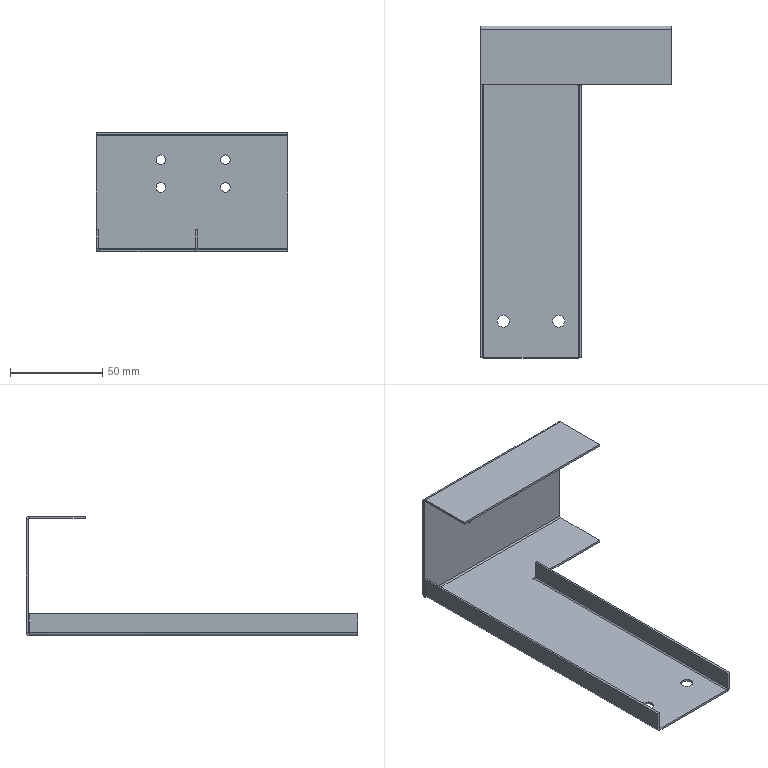Part | 1 solid | 54 faces | box 103.8 x 180 x 65 mm | volume 29196 mm3 | plane 34 | cylinder 20 | commonest cylinder face diameters 5.2 x8 1.473 x4 3.873 x4 6.5 x4
STEP:
#1=CARTESIAN_POINT('',(42.5,88.8,46.2));
#2=VERTEX_POINT('',#1);
#3=CARTESIAN_POINT('',(42.5,88.8,51.4));
#4=VERTEX_POINT('',#3);
#5=CARTESIAN_POINT('',(42.5,88.8,48.8));
#6=DIRECTION('',(0.,1.,0.));
#7=DIRECTION('',(0.,0.,1.));
#8=AXIS2_PLACEMENT_3D('',#5,#6,#7);
#9=CIRCLE('',#8,2.6);
#10=EDGE_CURVE('',#2,#4,#9,.T.);
#11=ORIENTED_EDGE('',*,*,#10,.F.);
#12=CARTESIAN_POINT('',(42.5,90.,46.2));
#13=VERTEX_POINT('',#12);
#14=CARTESIAN_POINT('',(42.5,80.,46.2));
#15=DIRECTION('',(0.,1.,0.));
#16=VECTOR('',#15,1000.);
#17=LINE('',#14,#16);
#18=EDGE_CURVE('',#2,#13,#17,.T.);
#19=ORIENTED_EDGE('',*,*,#18,.T.);
#20=CARTESIAN_POINT('',(42.5,90.,51.4));
#21=VERTEX_POINT('',#20);
#22=CARTESIAN_POINT('',(42.5,90.,48.8));
#23=DIRECTION('',(0.,1.,0.));
#24=DIRECTION('',(0.,0.,1.));
#25=AXIS2_PLACEMENT_3D('',#22,#23,#24);
#26=CIRCLE('',#25,2.6);
#27=EDGE_CURVE('',#13,#21,#26,.T.);
#28=ORIENTED_EDGE('',*,*,#27,.T.);
#29=CARTESIAN_POINT('',(42.5,80.,51.4));
#30=DIRECTION('',(0.,1.,0.));
#31=VECTOR('',#30,1000.);
#32=LINE('',#29,#31);
#33=EDGE_CURVE('',#4,#21,#32,.T.);
#34=ORIENTED_EDGE('',*,*,#33,.F.);
#35=EDGE_LOOP('',(#11,#19,#28,#34));
#36=FACE_OUTER_BOUND('',#35,.T.);
#37=CARTESIAN_POINT('',(42.5,80.,48.8));
#38=DIRECTION('',(0.,1.,0.));
#39=DIRECTION('',(0.,0.,1.));
#40=AXIS2_PLACEMENT_3D('',#37,#38,#39);
#41=CYLINDRICAL_SURFACE('',#40,2.6);
#42=ADVANCED_FACE('',(#36),#41,.F.);
#43=CARTESIAN_POINT('',(7.5,88.8,46.2));
#44=VERTEX_POINT('',#43);
#45=CARTESIAN_POINT('',(7.5,88.8,51.4));
#46=VERTEX_POINT('',#45);
#47=CARTESIAN_POINT('',(7.5,88.8,48.8));
#48=DIRECTION('',(0.,1.,0.));
#49=DIRECTION('',(0.,0.,1.));
#50=AXIS2_PLACEMENT_3D('',#47,#48,#49);
#51=CIRCLE('',#50,2.6);
#52=EDGE_CURVE('',#44,#46,#51,.T.);
#53=ORIENTED_EDGE('',*,*,#52,.F.);
#54=CARTESIAN_POINT('',(7.5,90.,46.2));
#55=VERTEX_POINT('',#54);
#56=CARTESIAN_POINT('',(7.5,80.,46.2));
#57=DIRECTION('',(0.,1.,0.));
#58=VECTOR('',#57,1000.);
#59=LINE('',#56,#58);
#60=EDGE_CURVE('',#44,#55,#59,.T.);
#61=ORIENTED_EDGE('',*,*,#60,.T.);
#62=CARTESIAN_POINT('',(7.5,90.,51.4));
#63=VERTEX_POINT('',#62);
#64=CARTESIAN_POINT('',(7.5,90.,48.8));
#65=DIRECTION('',(0.,1.,0.));
#66=DIRECTION('',(0.,0.,1.));
#67=AXIS2_PLACEMENT_3D('',#64,#65,#66);
#68=CIRCLE('',#67,2.6);
#69=EDGE_CURVE('',#55,#63,#68,.T.);
#70=ORIENTED_EDGE('',*,*,#69,.T.);
#71=CARTESIAN_POINT('',(7.5,80.,51.4));
#72=DIRECTION('',(0.,1.,0.));
#73=VECTOR('',#72,1000.);
#74=LINE('',#71,#73);
#75=EDGE_CURVE('',#46,#63,#74,.T.);
#76=ORIENTED_EDGE('',*,*,#75,.F.);
#77=EDGE_LOOP('',(#53,#61,#70,#76));
#78=FACE_OUTER_BOUND('',#77,.T.);
#79=CARTESIAN_POINT('',(7.5,80.,48.8));
#80=DIRECTION('',(0.,1.,0.));
#81=DIRECTION('',(0.,0.,1.));
#82=AXIS2_PLACEMENT_3D('',#79,#80,#81);
#83=CYLINDRICAL_SURFACE('',#82,2.6);
#84=ADVANCED_FACE('',(#78),#83,.F.);
#85=CARTESIAN_POINT('',(7.5,88.8,31.2));
#86=VERTEX_POINT('',#85);
#87=CARTESIAN_POINT('',(7.5,88.8,36.4));
#88=VERTEX_POINT('',#87);
#89=CARTESIAN_POINT('',(7.5,88.8,33.8));
#90=DIRECTION('',(0.,1.,0.));
#91=DIRECTION('',(0.,0.,1.));
#92=AXIS2_PLACEMENT_3D('',#89,#90,#91);
#93=CIRCLE('',#92,2.6);
#94=EDGE_CURVE('',#86,#88,#93,.T.);
#95=ORIENTED_EDGE('',*,*,#94,.F.);
#96=CARTESIAN_POINT('',(7.5,90.,31.2));
#97=VERTEX_POINT('',#96);
#98=CARTESIAN_POINT('',(7.5,80.,31.2));
#99=DIRECTION('',(0.,1.,0.));
#100=VECTOR('',#99,1000.);
#101=LINE('',#98,#100);
#102=EDGE_CURVE('',#86,#97,#101,.T.);
#103=ORIENTED_EDGE('',*,*,#102,.T.);
#104=CARTESIAN_POINT('',(7.5,90.,36.4));
#105=VERTEX_POINT('',#104);
#106=CARTESIAN_POINT('',(7.5,90.,33.8));
#107=DIRECTION('',(0.,1.,0.));
#108=DIRECTION('',(0.,0.,1.));
#109=AXIS2_PLACEMENT_3D('',#106,#107,#108);
#110=CIRCLE('',#109,2.6);
#111=EDGE_CURVE('',#97,#105,#110,.T.);
#112=ORIENTED_EDGE('',*,*,#111,.T.);
#113=CARTESIAN_POINT('',(7.5,80.,36.4));
#114=DIRECTION('',(0.,1.,0.));
#115=VECTOR('',#114,1000.);
#116=LINE('',#113,#115);
#117=EDGE_CURVE('',#88,#105,#116,.T.);
#118=ORIENTED_EDGE('',*,*,#117,.F.);
#119=EDGE_LOOP('',(#95,#103,#112,#118));
#120=FACE_OUTER_BOUND('',#119,.T.);
#121=CARTESIAN_POINT('',(7.5,80.,33.8));
#122=DIRECTION('',(0.,1.,0.));
#123=DIRECTION('',(0.,0.,1.));
#124=AXIS2_PLACEMENT_3D('',#121,#122,#123);
#125=CYLINDRICAL_SURFACE('',#124,2.6);
#126=ADVANCED_FACE('',(#120),#125,.F.);
#127=CARTESIAN_POINT('',(42.5,88.8,31.2));
#128=VERTEX_POINT('',#127);
#129=CARTESIAN_POINT('',(42.5,88.8,36.4));
#130=VERTEX_POINT('',#129);
#131=CARTESIAN_POINT('',(42.5,88.8,33.8));
#132=DIRECTION('',(0.,1.,0.));
#133=DIRECTION('',(0.,0.,1.));
#134=AXIS2_PLACEMENT_3D('',#131,#132,#133);
#135=CIRCLE('',#134,2.6);
#136=EDGE_CURVE('',#128,#130,#135,.T.);
#137=ORIENTED_EDGE('',*,*,#136,.F.);
#138=CARTESIAN_POINT('',(42.5,90.,31.2));
#139=VERTEX_POINT('',#138);
#140=CARTESIAN_POINT('',(42.5,80.,31.2));
#141=DIRECTION('',(0.,1.,0.));
#142=VECTOR('',#141,1000.);
#143=LINE('',#140,#142);
#144=EDGE_CURVE('',#128,#139,#143,.T.);
#145=ORIENTED_EDGE('',*,*,#144,.T.);
#146=CARTESIAN_POINT('',(42.5,90.,36.4));
#147=VERTEX_POINT('',#146);
#148=CARTESIAN_POINT('',(42.5,90.,33.8));
#149=DIRECTION('',(0.,1.,0.));
#150=DIRECTION('',(0.,0.,1.));
#151=AXIS2_PLACEMENT_3D('',#148,#149,#150);
#152=CIRCLE('',#151,2.6);
#153=EDGE_CURVE('',#139,#147,#152,.T.);
#154=ORIENTED_EDGE('',*,*,#153,.T.);
#155=CARTESIAN_POINT('',(42.5,80.,36.4));
#156=DIRECTION('',(0.,1.,0.));
#157=VECTOR('',#156,1000.);
#158=LINE('',#155,#157);
#159=EDGE_CURVE('',#130,#147,#158,.T.);
#160=ORIENTED_EDGE('',*,*,#159,.F.);
#161=EDGE_LOOP('',(#137,#145,#154,#160));
#162=FACE_OUTER_BOUND('',#161,.T.);
#163=CARTESIAN_POINT('',(42.5,80.,33.8));
#164=DIRECTION('',(0.,1.,0.));
#165=DIRECTION('',(0.,0.,1.));
#166=AXIS2_PLACEMENT_3D('',#163,#164,#165);
#167=CYLINDRICAL_SURFACE('',#166,2.6);
#168=ADVANCED_FACE('',(#162),#167,.F.);
#169=CARTESIAN_POINT('',(18.25,-70.,0.));
#170=VERTEX_POINT('',#169);
#171=CARTESIAN_POINT('',(11.75,-70.,0.));
#172=VERTEX_POINT('',#171);
#173=CARTESIAN_POINT('',(15.,-70.,0.));
#174=DIRECTION('',(0.,0.,-1.));
#175=DIRECTION('',(-1.,0.,0.));
#176=AXIS2_PLACEMENT_3D('',#173,#174,#175);
#177=CIRCLE('',#176,3.25);
#178=EDGE_CURVE('',#170,#172,#177,.T.);
#179=ORIENTED_EDGE('',*,*,#178,.F.);
#180=CARTESIAN_POINT('',(18.25,-70.,-1.2));
#181=VERTEX_POINT('',#180);
#182=CARTESIAN_POINT('',(18.25,-70.,8.8));
#183=DIRECTION('',(0.,0.,-1.));
#184=VECTOR('',#183,1000.);
#185=LINE('',#182,#184);
#186=EDGE_CURVE('',#170,#181,#185,.T.);
#187=ORIENTED_EDGE('',*,*,#186,.T.);
#188=CARTESIAN_POINT('',(11.75,-70.,-1.2));
#189=VERTEX_POINT('',#188);
#190=CARTESIAN_POINT('',(15.,-70.,-1.2));
#191=DIRECTION('',(0.,0.,-1.));
#192=DIRECTION('',(-1.,0.,0.));
#193=AXIS2_PLACEMENT_3D('',#190,#191,#192);
#194=CIRCLE('',#193,3.25);
#195=EDGE_CURVE('',#181,#189,#194,.T.);
#196=ORIENTED_EDGE('',*,*,#195,.T.);
#197=CARTESIAN_POINT('',(11.75,-70.,8.8));
#198=DIRECTION('',(0.,0.,-1.));
#199=VECTOR('',#198,1000.);
#200=LINE('',#197,#199);
#201=EDGE_CURVE('',#172,#189,#200,.T.);
#202=ORIENTED_EDGE('',*,*,#201,.F.);
#203=EDGE_LOOP('',(#179,#187,#196,#202));
#204=FACE_OUTER_BOUND('',#203,.T.);
#205=CARTESIAN_POINT('',(15.,-70.,8.8));
#206=DIRECTION('',(0.,0.,-1.));
#207=DIRECTION('',(-1.,0.,0.));
#208=AXIS2_PLACEMENT_3D('',#205,#206,#207);
#209=CYLINDRICAL_SURFACE('',#208,3.25);
#210=ADVANCED_FACE('',(#204),#209,.F.);
#211=CARTESIAN_POINT('',(-11.75,-70.,0.));
#212=VERTEX_POINT('',#211);
#213=CARTESIAN_POINT('',(-18.25,-70.,0.));
#214=VERTEX_POINT('',#213);
#215=CARTESIAN_POINT('',(-15.,-70.,0.));
#216=DIRECTION('',(0.,0.,-1.));
#217=DIRECTION('',(-1.,0.,0.));
#218=AXIS2_PLACEMENT_3D('',#215,#216,#217);
#219=CIRCLE('',#218,3.25);
#220=EDGE_CURVE('',#212,#214,#219,.T.);
#221=ORIENTED_EDGE('',*,*,#220,.F.);
#222=CARTESIAN_POINT('',(-11.75,-70.,-1.2));
#223=VERTEX_POINT('',#222);
#224=CARTESIAN_POINT('',(-11.75,-70.,8.8));
#225=DIRECTION('',(0.,0.,-1.));
#226=VECTOR('',#225,1000.);
#227=LINE('',#224,#226);
#228=EDGE_CURVE('',#212,#223,#227,.T.);
#229=ORIENTED_EDGE('',*,*,#228,.T.);
#230=CARTESIAN_POINT('',(-18.25,-70.,-1.2));
#231=VERTEX_POINT('',#230);
#232=CARTESIAN_POINT('',(-15.,-70.,-1.2));
#233=DIRECTION('',(0.,0.,-1.));
#234=DIRECTION('',(-1.,0.,0.));
#235=AXIS2_PLACEMENT_3D('',#232,#233,#234);
#236=CIRCLE('',#235,3.25);
#237=EDGE_CURVE('',#223,#231,#236,.T.);
#238=ORIENTED_EDGE('',*,*,#237,.T.);
#239=CARTESIAN_POINT('',(-18.25,-70.,8.8));
#240=DIRECTION('',(0.,0.,-1.));
#241=VECTOR('',#240,1000.);
#242=LINE('',#239,#241);
#243=EDGE_CURVE('',#214,#231,#242,.T.);
#244=ORIENTED_EDGE('',*,*,#243,.F.);
#245=EDGE_LOOP('',(#221,#229,#238,#244));
#246=FACE_OUTER_BOUND('',#245,.T.);
#247=CARTESIAN_POINT('',(-15.,-70.,8.8));
#248=DIRECTION('',(0.,0.,-1.));
#249=DIRECTION('',(-1.,0.,0.));
#250=AXIS2_PLACEMENT_3D('',#247,#248,#249);
#251=CYLINDRICAL_SURFACE('',#250,3.25);
#252=ADVANCED_FACE('',(#246),#251,.F.);
#253=CARTESIAN_POINT('',(-27.5,88.063,-1.2));
#254=VERTEX_POINT('',#253);
#255=CARTESIAN_POINT('',(-25.563,88.063,-1.2));
#256=VERTEX_POINT('',#255);
#257=CARTESIAN_POINT('',(-27.5,88.063,-1.2));
#258=DIRECTION('',(1.,0.,0.));
#259=VECTOR('',#258,1000.);
#260=LINE('',#257,#259);
#261=EDGE_CURVE('',#254,#256,#260,.T.);
#262=ORIENTED_EDGE('',*,*,#261,.T.);
#263=CARTESIAN_POINT('',(-27.354,88.063,0.));
#264=VERTEX_POINT('',#263);
#265=CARTESIAN_POINT('',(-25.563,88.063,0.7366));
#266=DIRECTION('',(0.,1.,0.));
#267=DIRECTION('',(0.,0.,-1.));
#268=AXIS2_PLACEMENT_3D('',#265,#266,#267);
#269=CIRCLE('',#268,1.937);
#270=EDGE_CURVE('',#256,#264,#269,.T.);
#271=ORIENTED_EDGE('',*,*,#270,.T.);
#272=CARTESIAN_POINT('',(-27.5,88.063,0.));
#273=VERTEX_POINT('',#272);
#274=CARTESIAN_POINT('',(-27.5,88.063,0.));
#275=DIRECTION('',(1.,0.,0.));
#276=VECTOR('',#275,1000.);
#277=LINE('',#274,#276);
#278=EDGE_CURVE('',#273,#264,#277,.T.);
#279=ORIENTED_EDGE('',*,*,#278,.F.);
#280=CARTESIAN_POINT('',(-27.5,88.063,0.));
#281=DIRECTION('',(0.,0.,-1.));
#282=VECTOR('',#281,1000.);
#283=LINE('',#280,#282);
#284=EDGE_CURVE('',#273,#254,#283,.T.);
#285=ORIENTED_EDGE('',*,*,#284,.T.);
#286=EDGE_LOOP('',(#262,#271,#279,#285));
#287=FACE_OUTER_BOUND('',#286,.T.);
#288=CARTESIAN_POINT('',(-25.563,88.063,0.));
#289=DIRECTION('',(0.,-1.,0.));
#290=DIRECTION('',(0.,0.,-1.));
#291=AXIS2_PLACEMENT_3D('',#288,#289,#290);
#292=PLANE('',#291);
#293=ADVANCED_FACE('',(#287),#292,.T.);
#294=CARTESIAN_POINT('',(15.,-70.,-1.2));
#295=DIRECTION('',(0.,0.,-1.));
#296=DIRECTION('',(-1.,0.,0.));
#297=AXIS2_PLACEMENT_3D('',#294,#295,#296);
#298=CIRCLE('',#297,3.25);
#299=EDGE_CURVE('',#189,#181,#298,.T.);
#300=ORIENTED_EDGE('',*,*,#299,.F.);
#301=ORIENTED_EDGE('',*,*,#195,.F.);
#302=EDGE_LOOP('',(#300,#301));
#303=FACE_BOUND('',#302,.T.);
#304=CARTESIAN_POINT('',(-15.,-70.,-1.2));
#305=DIRECTION('',(0.,0.,-1.));
#306=DIRECTION('',(-1.,0.,0.));
#307=AXIS2_PLACEMENT_3D('',#304,#305,#306);
#308=CIRCLE('',#307,3.25);
#309=EDGE_CURVE('',#231,#223,#308,.T.);
#310=ORIENTED_EDGE('',*,*,#309,.F.);
#311=ORIENTED_EDGE('',*,*,#237,.F.);
#312=EDGE_LOOP('',(#310,#311));
#313=FACE_BOUND('',#312,.T.);
#314=CARTESIAN_POINT('',(-25.563,-90.,-1.2));
#315=VERTEX_POINT('',#314);
#316=CARTESIAN_POINT('',(25.563,-90.,-1.2));
#317=VERTEX_POINT('',#316);
#318=CARTESIAN_POINT('',(-27.5,-90.,-1.2));
#319=DIRECTION('',(1.,0.,0.));
#320=VECTOR('',#319,1000.);
#321=LINE('',#318,#320);
#322=EDGE_CURVE('',#315,#317,#321,.T.);
#323=ORIENTED_EDGE('',*,*,#322,.F.);
#324=CARTESIAN_POINT('',(-25.563,-90.,-1.2));
#325=DIRECTION('',(0.,1.,0.));
#326=VECTOR('',#325,1000.);
#327=LINE('',#324,#326);
#328=EDGE_CURVE('',#315,#256,#327,.T.);
#329=ORIENTED_EDGE('',*,*,#328,.T.);
#330=CARTESIAN_POINT('',(76.3,88.063,-1.2));
#331=VERTEX_POINT('',#330);
#332=CARTESIAN_POINT('',(-27.5,88.063,-1.2));
#333=DIRECTION('',(1.,0.,0.));
#334=VECTOR('',#333,1000.);
#335=LINE('',#332,#334);
#336=EDGE_CURVE('',#256,#331,#335,.T.);
#337=ORIENTED_EDGE('',*,*,#336,.T.);
#338=CARTESIAN_POINT('',(76.3,58.2,-1.2));
#339=VERTEX_POINT('',#338);
#340=CARTESIAN_POINT('',(76.3,-90.,-1.2));
#341=DIRECTION('',(0.,1.,0.));
#342=VECTOR('',#341,1000.);
#343=LINE('',#340,#342);
#344=EDGE_CURVE('',#339,#331,#343,.T.);
#345=ORIENTED_EDGE('',*,*,#344,.F.);
#346=CARTESIAN_POINT('',(24.963,58.2,-1.2));
#347=VERTEX_POINT('',#346);
#348=CARTESIAN_POINT('',(0.,58.2,-1.2));
#349=DIRECTION('',(-1.,0.,0.));
#350=VECTOR('',#349,1000.);
#351=LINE('',#348,#350);
#352=EDGE_CURVE('',#339,#347,#351,.T.);
#353=ORIENTED_EDGE('',*,*,#352,.T.);
#354=CARTESIAN_POINT('',(24.963,57.6,-1.2));
#355=VERTEX_POINT('',#354);
#356=CARTESIAN_POINT('',(24.963,0.,-1.2));
#357=DIRECTION('',(0.,-1.,0.));
#358=VECTOR('',#357,1000.);
#359=LINE('',#356,#358);
#360=EDGE_CURVE('',#347,#355,#359,.T.);
#361=ORIENTED_EDGE('',*,*,#360,.T.);
#362=CARTESIAN_POINT('',(25.563,57.6,-1.2));
#363=VERTEX_POINT('',#362);
#364=CARTESIAN_POINT('',(0.,57.6,-1.2));
#365=DIRECTION('',(1.,0.,0.));
#366=VECTOR('',#365,1000.);
#367=LINE('',#364,#366);
#368=EDGE_CURVE('',#355,#363,#367,.T.);
#369=ORIENTED_EDGE('',*,*,#368,.T.);
#370=CARTESIAN_POINT('',(25.563,57.6,-1.2));
#371=DIRECTION('',(0.,-1.,0.));
#372=VECTOR('',#371,1000.);
#373=LINE('',#370,#372);
#374=EDGE_CURVE('',#363,#317,#373,.T.);
#375=ORIENTED_EDGE('',*,*,#374,.T.);
#376=EDGE_LOOP('',(#323,#329,#337,#345,#353,#361,#369,#375));
#377=FACE_OUTER_BOUND('',#376,.T.);
#378=CARTESIAN_POINT('',(0.,0.,-1.2));
#379=DIRECTION('',(0.,0.,-1.));
#380=DIRECTION('',(-1.,0.,0.));
#381=AXIS2_PLACEMENT_3D('',#378,#379,#380);
#382=PLANE('',#381);
#383=ADVANCED_FACE('',(#303,#313,#377),#382,.T.);
#384=CARTESIAN_POINT('',(15.,-70.,0.));
#385=DIRECTION('',(0.,0.,-1.));
#386=DIRECTION('',(-1.,0.,0.));
#387=AXIS2_PLACEMENT_3D('',#384,#385,#386);
#388=CIRCLE('',#387,3.25);
#389=EDGE_CURVE('',#172,#170,#388,.T.);
#390=ORIENTED_EDGE('',*,*,#389,.T.);
#391=ORIENTED_EDGE('',*,*,#178,.T.);
#392=EDGE_LOOP('',(#390,#391));
#393=FACE_BOUND('',#392,.T.);
#394=CARTESIAN_POINT('',(-15.,-70.,0.));
#395=DIRECTION('',(0.,0.,-1.));
#396=DIRECTION('',(-1.,0.,0.));
#397=AXIS2_PLACEMENT_3D('',#394,#395,#396);
#398=CIRCLE('',#397,3.25);
#399=EDGE_CURVE('',#214,#212,#398,.T.);
#400=ORIENTED_EDGE('',*,*,#399,.T.);
#401=ORIENTED_EDGE('',*,*,#220,.T.);
#402=EDGE_LOOP('',(#400,#401));
#403=FACE_BOUND('',#402,.T.);
#404=CARTESIAN_POINT('',(-25.563,-90.,0.));
#405=VERTEX_POINT('',#404);
#406=CARTESIAN_POINT('',(-25.563,88.063,0.));
#407=VERTEX_POINT('',#406);
#408=CARTESIAN_POINT('',(-25.563,-90.,0.));
#409=DIRECTION('',(0.,1.,0.));
#410=VECTOR('',#409,1000.);
#411=LINE('',#408,#410);
#412=EDGE_CURVE('',#405,#407,#411,.T.);
#413=ORIENTED_EDGE('',*,*,#412,.F.);
#414=CARTESIAN_POINT('',(25.563,-90.,0.));
#415=VERTEX_POINT('',#414);
#416=CARTESIAN_POINT('',(-27.5,-90.,0.));
#417=DIRECTION('',(1.,0.,0.));
#418=VECTOR('',#417,1000.);
#419=LINE('',#416,#418);
#420=EDGE_CURVE('',#405,#415,#419,.T.);
#421=ORIENTED_EDGE('',*,*,#420,.T.);
#422=CARTESIAN_POINT('',(25.563,57.6,0.));
#423=VERTEX_POINT('',#422);
#424=CARTESIAN_POINT('',(25.563,57.6,0.));
#425=DIRECTION('',(0.,-1.,0.));
#426=VECTOR('',#425,1000.);
#427=LINE('',#424,#426);
#428=EDGE_CURVE('',#423,#415,#427,.T.);
#429=ORIENTED_EDGE('',*,*,#428,.F.);
#430=CARTESIAN_POINT('',(24.963,57.6,0.));
#431=VERTEX_POINT('',#430);
#432=CARTESIAN_POINT('',(24.963,57.6,0.));
#433=DIRECTION('',(1.,0.,0.));
#434=VECTOR('',#433,1000.);
#435=LINE('',#432,#434);
#436=EDGE_CURVE('',#431,#423,#435,.T.);
#437=ORIENTED_EDGE('',*,*,#436,.F.);
#438=CARTESIAN_POINT('',(24.963,58.2,0.));
#439=VERTEX_POINT('',#438);
#440=CARTESIAN_POINT('',(24.963,58.2,0.));
#441=DIRECTION('',(0.,-1.,0.));
#442=VECTOR('',#441,1000.);
#443=LINE('',#440,#442);
#444=EDGE_CURVE('',#439,#431,#443,.T.);
#445=ORIENTED_EDGE('',*,*,#444,.F.);
#446=CARTESIAN_POINT('',(76.3,58.2,0.));
#447=VERTEX_POINT('',#446);
#448=CARTESIAN_POINT('',(27.5,58.2,0.));
#449=DIRECTION('',(-1.,0.,0.));
#450=VECTOR('',#449,1000.);
#451=LINE('',#448,#450);
#452=EDGE_CURVE('',#447,#439,#451,.T.);
#453=ORIENTED_EDGE('',*,*,#452,.F.);
#454=CARTESIAN_POINT('',(76.3,88.063,0.));
#455=VERTEX_POINT('',#454);
#456=CARTESIAN_POINT('',(76.3,-90.,0.));
#457=DIRECTION('',(0.,1.,0.));
#458=VECTOR('',#457,1000.);
#459=LINE('',#456,#458);
#460=EDGE_CURVE('',#447,#455,#459,.T.);
#461=ORIENTED_EDGE('',*,*,#460,.T.);
#462=CARTESIAN_POINT('',(-27.5,88.063,0.));
#463=DIRECTION('',(1.,0.,0.));
#464=VECTOR('',#463,1000.);
#465=LINE('',#462,#464);
#466=EDGE_CURVE('',#407,#455,#465,.T.);
#467=ORIENTED_EDGE('',*,*,#466,.F.);
#468=EDGE_LOOP('',(#413,#421,#429,#437,#445,#453,#461,#467));
#469=FACE_OUTER_BOUND('',#468,.T.);
#470=CARTESIAN_POINT('',(0.,0.,0.));
#471=DIRECTION('',(0.,0.,-1.));
#472=DIRECTION('',(-1.,0.,0.));
#473=AXIS2_PLACEMENT_3D('',#470,#471,#472);
#474=PLANE('',#473);
#475=ADVANCED_FACE('',(#393,#403,#469),#474,.F.);
#476=ORIENTED_EDGE('',*,*,#420,.F.);
#477=CARTESIAN_POINT('',(-25.563,-90.,0.));
#478=DIRECTION('',(0.,0.,-1.));
#479=VECTOR('',#478,1000.);
#480=LINE('',#477,#479);
#481=EDGE_CURVE('',#405,#315,#480,.T.);
#482=ORIENTED_EDGE('',*,*,#481,.T.);
#483=ORIENTED_EDGE('',*,*,#322,.T.);
#484=CARTESIAN_POINT('',(25.563,-90.,0.));
#485=DIRECTION('',(0.,0.,-1.));
#486=VECTOR('',#485,1000.);
#487=LINE('',#484,#486);
#488=EDGE_CURVE('',#415,#317,#487,.T.);
#489=ORIENTED_EDGE('',*,*,#488,.F.);
#490=EDGE_LOOP('',(#476,#482,#483,#489));
#491=FACE_OUTER_BOUND('',#490,.T.);
#492=CARTESIAN_POINT('',(-27.5,-90.,-1.2));
#493=DIRECTION('',(0.,-1.,0.));
#494=DIRECTION('',(0.,0.,-1.));
#495=AXIS2_PLACEMENT_3D('',#492,#493,#494);
#496=PLANE('',#495);
#497=ADVANCED_FACE('',(#491),#496,.T.);
#498=ORIENTED_EDGE('',*,*,#460,.F.);
#499=CARTESIAN_POINT('',(76.3,58.2,0.));
#500=DIRECTION('',(0.,0.,-1.));
#501=VECTOR('',#500,1000.);
#502=LINE('',#499,#501);
#503=EDGE_CURVE('',#447,#339,#502,.T.);
#504=ORIENTED_EDGE('',*,*,#503,.T.);
#505=ORIENTED_EDGE('',*,*,#344,.T.);
#506=CARTESIAN_POINT('',(76.3,88.063,0.));
#507=DIRECTION('',(0.,0.,-1.));
#508=VECTOR('',#507,1000.);
#509=LINE('',#506,#508);
#510=EDGE_CURVE('',#455,#331,#509,.T.);
#511=ORIENTED_EDGE('',*,*,#510,.F.);
#512=EDGE_LOOP('',(#498,#504,#505,#511));
#513=FACE_OUTER_BOUND('',#512,.T.);
#514=CARTESIAN_POINT('',(76.3,-90.,-1.2));
#515=DIRECTION('',(1.,0.,0.));
#516=DIRECTION('',(0.,0.,-1.));
#517=AXIS2_PLACEMENT_3D('',#514,#515,#516);
#518=PLANE('',#517);
#519=ADVANCED_FACE('',(#513),#518,.T.);
#520=CARTESIAN_POINT('',(-27.5,88.8,61.863));
#521=VERTEX_POINT('',#520);
#522=CARTESIAN_POINT('',(-27.5,88.8,0.7366));
#523=VERTEX_POINT('',#522);
#524=CARTESIAN_POINT('',(-27.5,88.8,0.));
#525=DIRECTION('',(0.,0.,-1.));
#526=VECTOR('',#525,1000.);
#527=LINE('',#524,#526);
#528=EDGE_CURVE('',#521,#523,#527,.T.);
#529=ORIENTED_EDGE('',*,*,#528,.F.);
#530=CARTESIAN_POINT('',(-27.5,90.,61.863));
#531=VERTEX_POINT('',#530);
#532=CARTESIAN_POINT('',(-27.5,88.8,61.863));
#533=DIRECTION('',(0.,1.,0.));
#534=VECTOR('',#533,1000.);
#535=LINE('',#532,#534);
#536=EDGE_CURVE('',#521,#531,#535,.T.);
#537=ORIENTED_EDGE('',*,*,#536,.T.);
#538=CARTESIAN_POINT('',(-27.5,90.,0.7366));
#539=VERTEX_POINT('',#538);
#540=CARTESIAN_POINT('',(-27.5,90.,0.));
#541=DIRECTION('',(0.,0.,-1.));
#542=VECTOR('',#541,1000.);
#543=LINE('',#540,#542);
#544=EDGE_CURVE('',#531,#539,#543,.T.);
#545=ORIENTED_EDGE('',*,*,#544,.T.);
#546=CARTESIAN_POINT('',(-27.5,88.8,0.7366));
#547=DIRECTION('',(0.,1.,0.));
#548=VECTOR('',#547,1000.);
#549=LINE('',#546,#548);
#550=EDGE_CURVE('',#523,#539,#549,.T.);
#551=ORIENTED_EDGE('',*,*,#550,.F.);
#552=EDGE_LOOP('',(#529,#537,#545,#551));
#553=FACE_OUTER_BOUND('',#552,.T.);
#554=CARTESIAN_POINT('',(-27.5,90.,0.));
#555=DIRECTION('',(-1.,0.,0.));
#556=DIRECTION('',(0.,0.,1.));
#557=AXIS2_PLACEMENT_3D('',#554,#555,#556);
#558=PLANE('',#557);
#559=ADVANCED_FACE('',(#553),#558,.T.);
#560=CARTESIAN_POINT('',(42.5,90.,48.8));
#561=DIRECTION('',(0.,1.,0.));
#562=DIRECTION('',(0.,0.,1.));
#563=AXIS2_PLACEMENT_3D('',#560,#561,#562);
#564=CIRCLE('',#563,2.6);
#565=EDGE_CURVE('',#21,#13,#564,.T.);
#566=ORIENTED_EDGE('',*,*,#565,.F.);
#567=ORIENTED_EDGE('',*,*,#27,.F.);
#568=EDGE_LOOP('',(#566,#567));
#569=FACE_BOUND('',#568,.T.);
#570=CARTESIAN_POINT('',(7.5,90.,48.8));
#571=DIRECTION('',(0.,1.,0.));
#572=DIRECTION('',(0.,0.,1.));
#573=AXIS2_PLACEMENT_3D('',#570,#571,#572);
#574=CIRCLE('',#573,2.6);
#575=EDGE_CURVE('',#63,#55,#574,.T.);
#576=ORIENTED_EDGE('',*,*,#575,.F.);
#577=ORIENTED_EDGE('',*,*,#69,.F.);
#578=EDGE_LOOP('',(#576,#577));
#579=FACE_BOUND('',#578,.T.);
#580=CARTESIAN_POINT('',(7.5,90.,33.8));
#581=DIRECTION('',(0.,1.,0.));
#582=DIRECTION('',(0.,0.,1.));
#583=AXIS2_PLACEMENT_3D('',#580,#581,#582);
#584=CIRCLE('',#583,2.6);
#585=EDGE_CURVE('',#105,#97,#584,.T.);
#586=ORIENTED_EDGE('',*,*,#585,.F.);
#587=ORIENTED_EDGE('',*,*,#111,.F.);
#588=EDGE_LOOP('',(#586,#587));
#589=FACE_BOUND('',#588,.T.);
#590=CARTESIAN_POINT('',(42.5,90.,33.8));
#591=DIRECTION('',(0.,1.,0.));
#592=DIRECTION('',(0.,0.,1.));
#593=AXIS2_PLACEMENT_3D('',#590,#591,#592);
#594=CIRCLE('',#593,2.6);
#595=EDGE_CURVE('',#147,#139,#594,.T.);
#596=ORIENTED_EDGE('',*,*,#595,.F.);
#597=ORIENTED_EDGE('',*,*,#153,.F.);
#598=EDGE_LOOP('',(#596,#597));
#599=FACE_BOUND('',#598,.T.);
#600=ORIENTED_EDGE('',*,*,#544,.F.);
#601=CARTESIAN_POINT('',(76.3,90.,61.863));
#602=VERTEX_POINT('',#601);
#603=CARTESIAN_POINT('',(-27.5,90.,61.863));
#604=DIRECTION('',(1.,0.,0.));
#605=VECTOR('',#604,1000.);
#606=LINE('',#603,#605);
#607=EDGE_CURVE('',#531,#602,#606,.T.);
#608=ORIENTED_EDGE('',*,*,#607,.T.);
#609=CARTESIAN_POINT('',(76.3,90.,0.7366));
#610=VERTEX_POINT('',#609);
#611=CARTESIAN_POINT('',(76.3,90.,63.8));
#612=DIRECTION('',(0.,0.,1.));
#613=VECTOR('',#612,1000.);
#614=LINE('',#611,#613);
#615=EDGE_CURVE('',#610,#602,#614,.T.);
#616=ORIENTED_EDGE('',*,*,#615,.F.);
#617=CARTESIAN_POINT('',(-27.5,90.,0.7366));
#618=DIRECTION('',(-1.,0.,0.));
#619=VECTOR('',#618,1000.);
#620=LINE('',#617,#619);
#621=EDGE_CURVE('',#610,#539,#620,.T.);
#622=ORIENTED_EDGE('',*,*,#621,.T.);
#623=EDGE_LOOP('',(#600,#608,#616,#622));
#624=FACE_OUTER_BOUND('',#623,.T.);
#625=CARTESIAN_POINT('',(0.,90.,0.));
#626=DIRECTION('',(0.,1.,0.));
#627=DIRECTION('',(0.,0.,1.));
#628=AXIS2_PLACEMENT_3D('',#625,#626,#627);
#629=PLANE('',#628);
#630=ADVANCED_FACE('',(#569,#579,#589,#599,#624),#629,.T.);
#631=CARTESIAN_POINT('',(42.5,88.8,48.8));
#632=DIRECTION('',(0.,1.,0.));
#633=DIRECTION('',(0.,0.,1.));
#634=AXIS2_PLACEMENT_3D('',#631,#632,#633);
#635=CIRCLE('',#634,2.6);
#636=EDGE_CURVE('',#4,#2,#635,.T.);
#637=ORIENTED_EDGE('',*,*,#636,.T.);
#638=ORIENTED_EDGE('',*,*,#10,.T.);
#639=EDGE_LOOP('',(#637,#638));
#640=FACE_BOUND('',#639,.T.);
#641=CARTESIAN_POINT('',(7.5,88.8,48.8));
#642=DIRECTION('',(0.,1.,0.));
#643=DIRECTION('',(0.,0.,1.));
#644=AXIS2_PLACEMENT_3D('',#641,#642,#643);
#645=CIRCLE('',#644,2.6);
#646=EDGE_CURVE('',#46,#44,#645,.T.);
#647=ORIENTED_EDGE('',*,*,#646,.T.);
#648=ORIENTED_EDGE('',*,*,#52,.T.);
#649=EDGE_LOOP('',(#647,#648));
#650=FACE_BOUND('',#649,.T.);
#651=CARTESIAN_POINT('',(7.5,88.8,33.8));
#652=DIRECTION('',(0.,1.,0.));
#653=DIRECTION('',(0.,0.,1.));
#654=AXIS2_PLACEMENT_3D('',#651,#652,#653);
#655=CIRCLE('',#654,2.6);
#656=EDGE_CURVE('',#88,#86,#655,.T.);
#657=ORIENTED_EDGE('',*,*,#656,.T.);
#658=ORIENTED_EDGE('',*,*,#94,.T.);
#659=EDGE_LOOP('',(#657,#658));
#660=FACE_BOUND('',#659,.T.);
#661=CARTESIAN_POINT('',(42.5,88.8,33.8));
#662=DIRECTION('',(0.,1.,0.));
#663=DIRECTION('',(0.,0.,1.));
#664=AXIS2_PLACEMENT_3D('',#661,#662,#663);
#665=CIRCLE('',#664,2.6);
#666=EDGE_CURVE('',#130,#128,#665,.T.);
#667=ORIENTED_EDGE('',*,*,#666,.T.);
#668=ORIENTED_EDGE('',*,*,#136,.T.);
#669=EDGE_LOOP('',(#667,#668));
#670=FACE_BOUND('',#669,.T.);
#671=CARTESIAN_POINT('',(76.3,88.8,61.863));
#672=VERTEX_POINT('',#671);
#673=CARTESIAN_POINT('',(-27.5,88.8,61.863));
#674=DIRECTION('',(1.,0.,0.));
#675=VECTOR('',#674,1000.);
#676=LINE('',#673,#675);
#677=EDGE_CURVE('',#521,#672,#676,.T.);
#678=ORIENTED_EDGE('',*,*,#677,.F.);
#679=ORIENTED_EDGE('',*,*,#528,.T.);
#680=CARTESIAN_POINT('',(76.3,88.8,0.7366));
#681=VERTEX_POINT('',#680);
#682=CARTESIAN_POINT('',(-27.5,88.8,0.7366));
#683=DIRECTION('',(-1.,0.,0.));
#684=VECTOR('',#683,1000.);
#685=LINE('',#682,#684);
#686=EDGE_CURVE('',#681,#523,#685,.T.);
#687=ORIENTED_EDGE('',*,*,#686,.F.);
#688=CARTESIAN_POINT('',(76.3,88.8,0.));
#689=DIRECTION('',(0.,0.,1.));
#690=VECTOR('',#689,1000.);
#691=LINE('',#688,#690);
#692=EDGE_CURVE('',#681,#672,#691,.T.);
#693=ORIENTED_EDGE('',*,*,#692,.T.);
#694=EDGE_LOOP('',(#678,#679,#687,#693));
#695=FACE_OUTER_BOUND('',#694,.T.);
#696=CARTESIAN_POINT('',(0.,88.8,0.));
#697=DIRECTION('',(0.,1.,0.));
#698=DIRECTION('',(0.,0.,1.));
#699=AXIS2_PLACEMENT_3D('',#696,#697,#698);
#700=PLANE('',#699);
#701=ADVANCED_FACE('',(#640,#650,#660,#670,#695),#700,.F.);
#702=CARTESIAN_POINT('',(76.3,88.063,0.7366));
#703=DIRECTION('',(1.,0.,0.));
#704=DIRECTION('',(0.,0.,1.));
#705=AXIS2_PLACEMENT_3D('',#702,#703,#704);
#706=CIRCLE('',#705,1.937);
#707=EDGE_CURVE('',#331,#610,#706,.T.);
#708=ORIENTED_EDGE('',*,*,#707,.T.);
#709=ORIENTED_EDGE('',*,*,#615,.T.);
#710=CARTESIAN_POINT('',(76.3,88.8,61.863));
#711=DIRECTION('',(0.,1.,0.));
#712=VECTOR('',#711,1000.);
#713=LINE('',#710,#712);
#714=EDGE_CURVE('',#672,#602,#713,.T.);
#715=ORIENTED_EDGE('',*,*,#714,.F.);
#716=ORIENTED_EDGE('',*,*,#692,.F.);
#717=CARTESIAN_POINT('',(76.3,88.063,0.7366));
#718=DIRECTION('',(1.,0.,0.));
#719=DIRECTION('',(0.,0.,1.));
#720=AXIS2_PLACEMENT_3D('',#717,#718,#719);
#721=CIRCLE('',#720,0.7366);
#722=EDGE_CURVE('',#455,#681,#721,.T.);
#723=ORIENTED_EDGE('',*,*,#722,.F.);
#724=ORIENTED_EDGE('',*,*,#510,.T.);
#725=EDGE_LOOP('',(#708,#709,#715,#716,#723,#724));
#726=FACE_OUTER_BOUND('',#725,.T.);
#727=CARTESIAN_POINT('',(76.3,88.063,0.7366));
#728=DIRECTION('',(1.,0.,0.));
#729=DIRECTION('',(0.,0.,-1.));
#730=AXIS2_PLACEMENT_3D('',#727,#728,#729);
#731=PLANE('',#730);
#732=ADVANCED_FACE('',(#726),#731,.T.);
#733=CARTESIAN_POINT('',(-27.5,88.063,0.7366));
#734=DIRECTION('',(-1.,0.,0.));
#735=DIRECTION('',(0.,0.,1.));
#736=AXIS2_PLACEMENT_3D('',#733,#734,#735);
#737=CIRCLE('',#736,0.7366);
#738=EDGE_CURVE('',#523,#273,#737,.T.);
#739=ORIENTED_EDGE('',*,*,#738,.F.);
#740=ORIENTED_EDGE('',*,*,#550,.T.);
#741=CARTESIAN_POINT('',(-27.5,88.063,0.7366));
#742=DIRECTION('',(-1.,0.,0.));
#743=DIRECTION('',(0.,0.,1.));
#744=AXIS2_PLACEMENT_3D('',#741,#742,#743);
#745=CIRCLE('',#744,1.937);
#746=EDGE_CURVE('',#539,#254,#745,.T.);
#747=ORIENTED_EDGE('',*,*,#746,.T.);
#748=ORIENTED_EDGE('',*,*,#284,.F.);
#749=EDGE_LOOP('',(#739,#740,#747,#748));
#750=FACE_OUTER_BOUND('',#749,.T.);
#751=CARTESIAN_POINT('',(-27.5,88.063,0.7366));
#752=DIRECTION('',(1.,0.,0.));
#753=DIRECTION('',(0.,0.,-1.));
#754=AXIS2_PLACEMENT_3D('',#751,#752,#753);
#755=PLANE('',#754);
#756=ADVANCED_FACE('',(#750),#755,.F.);
#757=ORIENTED_EDGE('',*,*,#261,.F.);
#758=ORIENTED_EDGE('',*,*,#746,.F.);
#759=ORIENTED_EDGE('',*,*,#621,.F.);
#760=ORIENTED_EDGE('',*,*,#707,.F.);
#761=ORIENTED_EDGE('',*,*,#336,.F.);
#762=EDGE_LOOP('',(#757,#758,#759,#760,#761));
#763=FACE_OUTER_BOUND('',#762,.T.);
#764=CARTESIAN_POINT('',(-27.5,88.063,0.7366));
#765=DIRECTION('',(-1.,0.,0.));
#766=DIRECTION('',(0.,1.,0.));
#767=AXIS2_PLACEMENT_3D('',#764,#765,#766);
#768=CYLINDRICAL_SURFACE('',#767,1.937);
#769=ADVANCED_FACE('',(#763),#768,.T.);
#770=ORIENTED_EDGE('',*,*,#278,.T.);
#771=CARTESIAN_POINT('',(-27.5,88.063,0.));
#772=DIRECTION('',(1.,0.,0.));
#773=VECTOR('',#772,1000.);
#774=LINE('',#771,#773);
#775=EDGE_CURVE('',#264,#407,#774,.T.);
#776=ORIENTED_EDGE('',*,*,#775,.T.);
#777=ORIENTED_EDGE('',*,*,#466,.T.);
#778=ORIENTED_EDGE('',*,*,#722,.T.);
#779=ORIENTED_EDGE('',*,*,#686,.T.);
#780=ORIENTED_EDGE('',*,*,#738,.T.);
#781=EDGE_LOOP('',(#770,#776,#777,#778,#779,#780));
#782=FACE_OUTER_BOUND('',#781,.T.);
#783=CARTESIAN_POINT('',(-27.5,88.063,0.7366));
#784=DIRECTION('',(-1.,0.,0.));
#785=DIRECTION('',(0.,1.,0.));
#786=AXIS2_PLACEMENT_3D('',#783,#784,#785);
#787=CYLINDRICAL_SURFACE('',#786,0.7366);
#788=ADVANCED_FACE('',(#782),#787,.F.);
#789=CARTESIAN_POINT('',(76.3,88.063,62.6));
#790=VERTEX_POINT('',#789);
#791=CARTESIAN_POINT('',(76.3,88.063,63.8));
#792=VERTEX_POINT('',#791);
#793=CARTESIAN_POINT('',(76.3,88.063,63.8));
#794=DIRECTION('',(0.,0.,1.));
#795=VECTOR('',#794,1000.);
#796=LINE('',#793,#795);
#797=EDGE_CURVE('',#790,#792,#796,.T.);
#798=ORIENTED_EDGE('',*,*,#797,.F.);
#799=CARTESIAN_POINT('',(76.3,88.063,61.863));
#800=DIRECTION('',(1.,0.,0.));
#801=DIRECTION('',(0.,0.,1.));
#802=AXIS2_PLACEMENT_3D('',#799,#800,#801);
#803=CIRCLE('',#802,0.7366);
#804=EDGE_CURVE('',#672,#790,#803,.T.);
#805=ORIENTED_EDGE('',*,*,#804,.F.);
#806=ORIENTED_EDGE('',*,*,#714,.T.);
#807=CARTESIAN_POINT('',(76.3,88.063,61.863));
#808=DIRECTION('',(1.,0.,0.));
#809=DIRECTION('',(0.,0.,1.));
#810=AXIS2_PLACEMENT_3D('',#807,#808,#809);
#811=CIRCLE('',#810,1.937);
#812=EDGE_CURVE('',#602,#792,#811,.T.);
#813=ORIENTED_EDGE('',*,*,#812,.T.);
#814=EDGE_LOOP('',(#798,#805,#806,#813));
#815=FACE_OUTER_BOUND('',#814,.T.);
#816=CARTESIAN_POINT('',(76.3,88.063,61.863));
#817=DIRECTION('',(1.,0.,0.));
#818=DIRECTION('',(0.,0.,-1.));
#819=AXIS2_PLACEMENT_3D('',#816,#817,#818);
#820=PLANE('',#819);
#821=ADVANCED_FACE('',(#815),#820,.T.);
#822=CARTESIAN_POINT('',(-27.5,88.063,62.6));
#823=VERTEX_POINT('',#822);
#824=CARTESIAN_POINT('',(-27.5,88.063,61.863));
#825=DIRECTION('',(-1.,0.,0.));
#826=DIRECTION('',(0.,0.,1.));
#827=AXIS2_PLACEMENT_3D('',#824,#825,#826);
#828=CIRCLE('',#827,0.7366);
#829=EDGE_CURVE('',#823,#521,#828,.T.);
#830=ORIENTED_EDGE('',*,*,#829,.F.);
#831=CARTESIAN_POINT('',(-27.5,88.063,63.8));
#832=VERTEX_POINT('',#831);
#833=CARTESIAN_POINT('',(-27.5,88.063,62.6));
#834=DIRECTION('',(0.,0.,1.));
#835=VECTOR('',#834,1000.);
#836=LINE('',#833,#835);
#837=EDGE_CURVE('',#823,#832,#836,.T.);
#838=ORIENTED_EDGE('',*,*,#837,.T.);
#839=CARTESIAN_POINT('',(-27.5,88.063,61.863));
#840=DIRECTION('',(-1.,0.,0.));
#841=DIRECTION('',(0.,0.,1.));
#842=AXIS2_PLACEMENT_3D('',#839,#840,#841);
#843=CIRCLE('',#842,1.937);
#844=EDGE_CURVE('',#832,#531,#843,.T.);
#845=ORIENTED_EDGE('',*,*,#844,.T.);
#846=ORIENTED_EDGE('',*,*,#536,.F.);
#847=EDGE_LOOP('',(#830,#838,#845,#846));
#848=FACE_OUTER_BOUND('',#847,.T.);
#849=CARTESIAN_POINT('',(-27.5,88.063,61.863));
#850=DIRECTION('',(1.,0.,0.));
#851=DIRECTION('',(0.,0.,-1.));
#852=AXIS2_PLACEMENT_3D('',#849,#850,#851);
#853=PLANE('',#852);
#854=ADVANCED_FACE('',(#848),#853,.F.);
#855=ORIENTED_EDGE('',*,*,#607,.F.);
#856=ORIENTED_EDGE('',*,*,#844,.F.);
#857=CARTESIAN_POINT('',(0.,88.063,63.8));
#858=DIRECTION('',(-1.,0.,0.));
#859=VECTOR('',#858,1000.);
#860=LINE('',#857,#859);
#861=EDGE_CURVE('',#792,#832,#860,.T.);
#862=ORIENTED_EDGE('',*,*,#861,.F.);
#863=ORIENTED_EDGE('',*,*,#812,.F.);
#864=EDGE_LOOP('',(#855,#856,#862,#863));
#865=FACE_OUTER_BOUND('',#864,.T.);
#866=CARTESIAN_POINT('',(-27.5,88.063,61.863));
#867=DIRECTION('',(-1.,0.,0.));
#868=DIRECTION('',(0.,0.,1.));
#869=AXIS2_PLACEMENT_3D('',#866,#867,#868);
#870=CYLINDRICAL_SURFACE('',#869,1.937);
#871=ADVANCED_FACE('',(#865),#870,.T.);
#872=ORIENTED_EDGE('',*,*,#677,.T.);
#873=ORIENTED_EDGE('',*,*,#804,.T.);
#874=CARTESIAN_POINT('',(76.3,88.063,62.6));
#875=DIRECTION('',(-1.,0.,0.));
#876=VECTOR('',#875,1000.);
#877=LINE('',#874,#876);
#878=EDGE_CURVE('',#790,#823,#877,.T.);
#879=ORIENTED_EDGE('',*,*,#878,.T.);
#880=ORIENTED_EDGE('',*,*,#829,.T.);
#881=EDGE_LOOP('',(#872,#873,#879,#880));
#882=FACE_OUTER_BOUND('',#881,.T.);
#883=CARTESIAN_POINT('',(-27.5,88.063,61.863));
#884=DIRECTION('',(-1.,0.,0.));
#885=DIRECTION('',(0.,0.,1.));
#886=AXIS2_PLACEMENT_3D('',#883,#884,#885);
#887=CYLINDRICAL_SURFACE('',#886,0.7366);
#888=ADVANCED_FACE('',(#882),#887,.F.);
#889=CARTESIAN_POINT('',(-27.5,58.,63.8));
#890=VERTEX_POINT('',#889);
#891=CARTESIAN_POINT('',(-27.5,88.8,63.8));
#892=DIRECTION('',(0.,1.,0.));
#893=VECTOR('',#892,1000.);
#894=LINE('',#891,#893);
#895=EDGE_CURVE('',#890,#832,#894,.T.);
#896=ORIENTED_EDGE('',*,*,#895,.T.);
#897=ORIENTED_EDGE('',*,*,#837,.F.);
#898=CARTESIAN_POINT('',(-27.5,58.,62.6));
#899=VERTEX_POINT('',#898);
#900=CARTESIAN_POINT('',(-27.5,0.,62.6));
#901=DIRECTION('',(0.,1.,0.));
#902=VECTOR('',#901,1000.);
#903=LINE('',#900,#902);
#904=EDGE_CURVE('',#899,#823,#903,.T.);
#905=ORIENTED_EDGE('',*,*,#904,.F.);
#906=CARTESIAN_POINT('',(-27.5,58.,63.8));
#907=DIRECTION('',(0.,0.,-1.));
#908=VECTOR('',#907,1000.);
#909=LINE('',#906,#908);
#910=EDGE_CURVE('',#890,#899,#909,.T.);
#911=ORIENTED_EDGE('',*,*,#910,.F.);
#912=EDGE_LOOP('',(#896,#897,#905,#911));
#913=FACE_OUTER_BOUND('',#912,.T.);
#914=CARTESIAN_POINT('',(-27.5,88.8,63.8));
#915=DIRECTION('',(-1.,0.,0.));
#916=DIRECTION('',(0.,0.,1.));
#917=AXIS2_PLACEMENT_3D('',#914,#915,#916);
#918=PLANE('',#917);
#919=ADVANCED_FACE('',(#913),#918,.T.);
#920=CARTESIAN_POINT('',(76.3,58.,62.6));
#921=VERTEX_POINT('',#920);
#922=CARTESIAN_POINT('',(76.3,0.,62.6));
#923=DIRECTION('',(0.,-1.,0.));
#924=VECTOR('',#923,1000.);
#925=LINE('',#922,#924);
#926=EDGE_CURVE('',#790,#921,#925,.T.);
#927=ORIENTED_EDGE('',*,*,#926,.F.);
#928=ORIENTED_EDGE('',*,*,#797,.T.);
#929=CARTESIAN_POINT('',(76.3,58.,63.8));
#930=VERTEX_POINT('',#929);
#931=CARTESIAN_POINT('',(76.3,58.,63.8));
#932=DIRECTION('',(0.,-1.,0.));
#933=VECTOR('',#932,1000.);
#934=LINE('',#931,#933);
#935=EDGE_CURVE('',#792,#930,#934,.T.);
#936=ORIENTED_EDGE('',*,*,#935,.T.);
#937=CARTESIAN_POINT('',(76.3,58.,63.8));
#938=DIRECTION('',(0.,0.,-1.));
#939=VECTOR('',#938,1000.);
#940=LINE('',#937,#939);
#941=EDGE_CURVE('',#930,#921,#940,.T.);
#942=ORIENTED_EDGE('',*,*,#941,.T.);
#943=EDGE_LOOP('',(#927,#928,#936,#942));
#944=FACE_OUTER_BOUND('',#943,.T.);
#945=CARTESIAN_POINT('',(76.3,58.,63.8));
#946=DIRECTION('',(1.,0.,0.));
#947=DIRECTION('',(0.,0.,-1.));
#948=AXIS2_PLACEMENT_3D('',#945,#946,#947);
#949=PLANE('',#948);
#950=ADVANCED_FACE('',(#944),#949,.T.);
#951=ORIENTED_EDGE('',*,*,#935,.F.);
#952=ORIENTED_EDGE('',*,*,#861,.T.);
#953=ORIENTED_EDGE('',*,*,#895,.F.);
#954=CARTESIAN_POINT('',(-27.5,58.,63.8));
#955=DIRECTION('',(-1.,0.,0.));
#956=VECTOR('',#955,1000.);
#957=LINE('',#954,#956);
#958=EDGE_CURVE('',#930,#890,#957,.T.);
#959=ORIENTED_EDGE('',*,*,#958,.F.);
#960=EDGE_LOOP('',(#951,#952,#953,#959));
#961=FACE_OUTER_BOUND('',#960,.T.);
#962=CARTESIAN_POINT('',(0.,0.,63.8));
#963=DIRECTION('',(0.,0.,1.));
#964=DIRECTION('',(0.,-1.,0.));
#965=AXIS2_PLACEMENT_3D('',#962,#963,#964);
#966=PLANE('',#965);
#967=ADVANCED_FACE('',(#961),#966,.T.);
#968=ORIENTED_EDGE('',*,*,#878,.F.);
#969=ORIENTED_EDGE('',*,*,#926,.T.);
#970=CARTESIAN_POINT('',(0.,58.,62.6));
#971=DIRECTION('',(-1.,0.,0.));
#972=VECTOR('',#971,1000.);
#973=LINE('',#970,#972);
#974=EDGE_CURVE('',#921,#899,#973,.T.);
#975=ORIENTED_EDGE('',*,*,#974,.T.);
#976=ORIENTED_EDGE('',*,*,#904,.T.);
#977=EDGE_LOOP('',(#968,#969,#975,#976));
#978=FACE_OUTER_BOUND('',#977,.T.);
#979=CARTESIAN_POINT('',(0.,0.,62.6));
#980=DIRECTION('',(0.,0.,1.));
#981=DIRECTION('',(0.,-1.,0.));
#982=AXIS2_PLACEMENT_3D('',#979,#980,#981);
#983=PLANE('',#982);
#984=ADVANCED_FACE('',(#978),#983,.F.);
#985=ORIENTED_EDGE('',*,*,#974,.F.);
#986=ORIENTED_EDGE('',*,*,#941,.F.);
#987=ORIENTED_EDGE('',*,*,#958,.T.);
#988=ORIENTED_EDGE('',*,*,#910,.T.);
#989=EDGE_LOOP('',(#985,#986,#987,#988));
#990=FACE_OUTER_BOUND('',#989,.T.);
#991=CARTESIAN_POINT('',(-27.5,58.,63.8));
#992=DIRECTION('',(0.,-1.,0.));
#993=DIRECTION('',(0.,0.,-1.));
#994=AXIS2_PLACEMENT_3D('',#991,#992,#993);
#995=PLANE('',#994);
#996=ADVANCED_FACE('',(#990),#995,.T.);
#997=ORIENTED_EDGE('',*,*,#228,.F.);
#998=ORIENTED_EDGE('',*,*,#399,.F.);
#999=ORIENTED_EDGE('',*,*,#243,.T.);
#1000=ORIENTED_EDGE('',*,*,#309,.T.);
#1001=EDGE_LOOP('',(#997,#998,#999,#1000));
#1002=FACE_OUTER_BOUND('',#1001,.T.);
#1003=CARTESIAN_POINT('',(-15.,-70.,8.8));
#1004=DIRECTION('',(0.,0.,-1.));
#1005=DIRECTION('',(-1.,0.,0.));
#1006=AXIS2_PLACEMENT_3D('',#1003,#1004,#1005);
#1007=CYLINDRICAL_SURFACE('',#1006,3.25);
#1008=ADVANCED_FACE('',(#1002),#1007,.F.);
#1009=ORIENTED_EDGE('',*,*,#186,.F.);
#1010=ORIENTED_EDGE('',*,*,#389,.F.);
#1011=ORIENTED_EDGE('',*,*,#201,.T.);
#1012=ORIENTED_EDGE('',*,*,#299,.T.);
#1013=EDGE_LOOP('',(#1009,#1010,#1011,#1012));
#1014=FACE_OUTER_BOUND('',#1013,.T.);
#1015=CARTESIAN_POINT('',(15.,-70.,8.8));
#1016=DIRECTION('',(0.,0.,-1.));
#1017=DIRECTION('',(-1.,0.,0.));
#1018=AXIS2_PLACEMENT_3D('',#1015,#1016,#1017);
#1019=CYLINDRICAL_SURFACE('',#1018,3.25);
#1020=ADVANCED_FACE('',(#1014),#1019,.F.);
#1021=ORIENTED_EDGE('',*,*,#144,.F.);
#1022=ORIENTED_EDGE('',*,*,#666,.F.);
#1023=ORIENTED_EDGE('',*,*,#159,.T.);
#1024=ORIENTED_EDGE('',*,*,#595,.T.);
#1025=EDGE_LOOP('',(#1021,#1022,#1023,#1024));
#1026=FACE_OUTER_BOUND('',#1025,.T.);
#1027=CARTESIAN_POINT('',(42.5,80.,33.8));
#1028=DIRECTION('',(0.,1.,0.));
#1029=DIRECTION('',(0.,0.,1.));
#1030=AXIS2_PLACEMENT_3D('',#1027,#1028,#1029);
#1031=CYLINDRICAL_SURFACE('',#1030,2.6);
#1032=ADVANCED_FACE('',(#1026),#1031,.F.);
#1033=ORIENTED_EDGE('',*,*,#102,.F.);
#1034=ORIENTED_EDGE('',*,*,#656,.F.);
#1035=ORIENTED_EDGE('',*,*,#117,.T.);
#1036=ORIENTED_EDGE('',*,*,#585,.T.);
#1037=EDGE_LOOP('',(#1033,#1034,#1035,#1036));
#1038=FACE_OUTER_BOUND('',#1037,.T.);
#1039=CARTESIAN_POINT('',(7.5,80.,33.8));
#1040=DIRECTION('',(0.,1.,0.));
#1041=DIRECTION('',(0.,0.,1.));
#1042=AXIS2_PLACEMENT_3D('',#1039,#1040,#1041);
#1043=CYLINDRICAL_SURFACE('',#1042,2.6);
#1044=ADVANCED_FACE('',(#1038),#1043,.F.);
#1045=ORIENTED_EDGE('',*,*,#60,.F.);
#1046=ORIENTED_EDGE('',*,*,#646,.F.);
#1047=ORIENTED_EDGE('',*,*,#75,.T.);
#1048=ORIENTED_EDGE('',*,*,#575,.T.);
#1049=EDGE_LOOP('',(#1045,#1046,#1047,#1048));
#1050=FACE_OUTER_BOUND('',#1049,.T.);
#1051=CARTESIAN_POINT('',(7.5,80.,48.8));
#1052=DIRECTION('',(0.,1.,0.));
#1053=DIRECTION('',(0.,0.,1.));
#1054=AXIS2_PLACEMENT_3D('',#1051,#1052,#1053);
#1055=CYLINDRICAL_SURFACE('',#1054,2.6);
#1056=ADVANCED_FACE('',(#1050),#1055,.F.);
#1057=ORIENTED_EDGE('',*,*,#18,.F.);
#1058=ORIENTED_EDGE('',*,*,#636,.F.);
#1059=ORIENTED_EDGE('',*,*,#33,.T.);
#1060=ORIENTED_EDGE('',*,*,#565,.T.);
#1061=EDGE_LOOP('',(#1057,#1058,#1059,#1060));
#1062=FACE_OUTER_BOUND('',#1061,.T.);
#1063=CARTESIAN_POINT('',(42.5,80.,48.8));
#1064=DIRECTION('',(0.,1.,0.));
#1065=DIRECTION('',(0.,0.,1.));
#1066=AXIS2_PLACEMENT_3D('',#1063,#1064,#1065);
#1067=CYLINDRICAL_SURFACE('',#1066,2.6);
#1068=ADVANCED_FACE('',(#1062),#1067,.F.);
#1069=ORIENTED_EDGE('',*,*,#352,.F.);
#1070=ORIENTED_EDGE('',*,*,#503,.F.);
#1071=ORIENTED_EDGE('',*,*,#452,.T.);
#1072=CARTESIAN_POINT('',(24.963,58.2,0.));
#1073=DIRECTION('',(0.,0.,-1.));
#1074=VECTOR('',#1073,1000.);
#1075=LINE('',#1072,#1074);
#1076=EDGE_CURVE('',#439,#347,#1075,.T.);
#1077=ORIENTED_EDGE('',*,*,#1076,.T.);
#1078=EDGE_LOOP('',(#1069,#1070,#1071,#1077));
#1079=FACE_OUTER_BOUND('',#1078,.T.);
#1080=CARTESIAN_POINT('',(27.5,58.2,0.));
#1081=DIRECTION('',(0.,-1.,0.));
#1082=DIRECTION('',(1.,0.,0.));
#1083=AXIS2_PLACEMENT_3D('',#1080,#1081,#1082);
#1084=PLANE('',#1083);
#1085=ADVANCED_FACE('',(#1079),#1084,.T.);
#1086=ORIENTED_EDGE('',*,*,#360,.F.);
#1087=ORIENTED_EDGE('',*,*,#1076,.F.);
#1088=ORIENTED_EDGE('',*,*,#444,.T.);
#1089=CARTESIAN_POINT('',(24.963,57.6,0.));
#1090=DIRECTION('',(0.,0.,-1.));
#1091=VECTOR('',#1090,1000.);
#1092=LINE('',#1089,#1091);
#1093=EDGE_CURVE('',#431,#355,#1092,.T.);
#1094=ORIENTED_EDGE('',*,*,#1093,.T.);
#1095=EDGE_LOOP('',(#1086,#1087,#1088,#1094));
#1096=FACE_OUTER_BOUND('',#1095,.T.);
#1097=CARTESIAN_POINT('',(24.963,58.2,0.));
#1098=DIRECTION('',(1.,0.,0.));
#1099=DIRECTION('',(0.,0.,-1.));
#1100=AXIS2_PLACEMENT_3D('',#1097,#1098,#1099);
#1101=PLANE('',#1100);
#1102=ADVANCED_FACE('',(#1096),#1101,.T.);
#1103=ORIENTED_EDGE('',*,*,#368,.F.);
#1104=ORIENTED_EDGE('',*,*,#1093,.F.);
#1105=ORIENTED_EDGE('',*,*,#436,.T.);
#1106=CARTESIAN_POINT('',(25.563,57.6,0.));
#1107=DIRECTION('',(0.,0.,-1.));
#1108=VECTOR('',#1107,1000.);
#1109=LINE('',#1106,#1108);
#1110=EDGE_CURVE('',#423,#363,#1109,.T.);
#1111=ORIENTED_EDGE('',*,*,#1110,.T.);
#1112=EDGE_LOOP('',(#1103,#1104,#1105,#1111));
#1113=FACE_OUTER_BOUND('',#1112,.T.);
#1114=CARTESIAN_POINT('',(24.963,57.6,0.));
#1115=DIRECTION('',(0.,1.,0.));
#1116=DIRECTION('',(0.,0.,1.));
#1117=AXIS2_PLACEMENT_3D('',#1114,#1115,#1116);
#1118=PLANE('',#1117);
#1119=ADVANCED_FACE('',(#1113),#1118,.T.);
#1120=CARTESIAN_POINT('',(26.3,-90.,0.7366));
#1121=VERTEX_POINT('',#1120);
#1122=CARTESIAN_POINT('',(27.5,-90.,0.7366));
#1123=VERTEX_POINT('',#1122);
#1124=CARTESIAN_POINT('',(27.5,-90.,0.7366));
#1125=DIRECTION('',(1.,0.,0.));
#1126=VECTOR('',#1125,1000.);
#1127=LINE('',#1124,#1126);
#1128=EDGE_CURVE('',#1121,#1123,#1127,.T.);
#1129=ORIENTED_EDGE('',*,*,#1128,.F.);
#1130=CARTESIAN_POINT('',(25.563,-90.,0.7366));
#1131=DIRECTION('',(0.,-1.,0.));
#1132=DIRECTION('',(0.,0.,1.));
#1133=AXIS2_PLACEMENT_3D('',#1130,#1131,#1132);
#1134=CIRCLE('',#1133,0.7366);
#1135=EDGE_CURVE('',#415,#1121,#1134,.T.);
#1136=ORIENTED_EDGE('',*,*,#1135,.F.);
#1137=ORIENTED_EDGE('',*,*,#488,.T.);
#1138=CARTESIAN_POINT('',(25.563,-90.,0.7366));
#1139=DIRECTION('',(0.,-1.,0.));
#1140=DIRECTION('',(0.,0.,1.));
#1141=AXIS2_PLACEMENT_3D('',#1138,#1139,#1140);
#1142=CIRCLE('',#1141,1.937);
#1143=EDGE_CURVE('',#317,#1123,#1142,.T.);
#1144=ORIENTED_EDGE('',*,*,#1143,.T.);
#1145=EDGE_LOOP('',(#1129,#1136,#1137,#1144));
#1146=FACE_OUTER_BOUND('',#1145,.T.);
#1147=CARTESIAN_POINT('',(25.563,-90.,0.7366));
#1148=DIRECTION('',(0.,-1.,0.));
#1149=DIRECTION('',(0.,0.,-1.));
#1150=AXIS2_PLACEMENT_3D('',#1147,#1148,#1149);
#1151=PLANE('',#1150);
#1152=ADVANCED_FACE('',(#1146),#1151,.T.);
#1153=CARTESIAN_POINT('',(26.3,57.6,0.7366));
#1154=VERTEX_POINT('',#1153);
#1155=CARTESIAN_POINT('',(25.563,57.6,0.7366));
#1156=DIRECTION('',(0.,1.,0.));
#1157=DIRECTION('',(0.,0.,1.));
#1158=AXIS2_PLACEMENT_3D('',#1155,#1156,#1157);
#1159=CIRCLE('',#1158,0.7366);
#1160=EDGE_CURVE('',#1154,#423,#1159,.T.);
#1161=ORIENTED_EDGE('',*,*,#1160,.F.);
#1162=CARTESIAN_POINT('',(27.5,57.6,0.7366));
#1163=VERTEX_POINT('',#1162);
#1164=CARTESIAN_POINT('',(26.3,57.6,0.7366));
#1165=DIRECTION('',(1.,0.,0.));
#1166=VECTOR('',#1165,1000.);
#1167=LINE('',#1164,#1166);
#1168=EDGE_CURVE('',#1154,#1163,#1167,.T.);
#1169=ORIENTED_EDGE('',*,*,#1168,.T.);
#1170=CARTESIAN_POINT('',(25.563,57.6,0.7366));
#1171=DIRECTION('',(0.,1.,0.));
#1172=DIRECTION('',(0.,0.,1.));
#1173=AXIS2_PLACEMENT_3D('',#1170,#1171,#1172);
#1174=CIRCLE('',#1173,1.937);
#1175=EDGE_CURVE('',#1163,#363,#1174,.T.);
#1176=ORIENTED_EDGE('',*,*,#1175,.T.);
#1177=ORIENTED_EDGE('',*,*,#1110,.F.);
#1178=EDGE_LOOP('',(#1161,#1169,#1176,#1177));
#1179=FACE_OUTER_BOUND('',#1178,.T.);
#1180=CARTESIAN_POINT('',(25.563,57.6,0.7366));
#1181=DIRECTION('',(0.,-1.,0.));
#1182=DIRECTION('',(0.,0.,-1.));
#1183=AXIS2_PLACEMENT_3D('',#1180,#1181,#1182);
#1184=PLANE('',#1183);
#1185=ADVANCED_FACE('',(#1179),#1184,.F.);
#1186=ORIENTED_EDGE('',*,*,#374,.F.);
#1187=ORIENTED_EDGE('',*,*,#1175,.F.);
#1188=CARTESIAN_POINT('',(27.5,0.,0.7366));
#1189=DIRECTION('',(0.,1.,0.));
#1190=VECTOR('',#1189,1000.);
#1191=LINE('',#1188,#1190);
#1192=EDGE_CURVE('',#1123,#1163,#1191,.T.);
#1193=ORIENTED_EDGE('',*,*,#1192,.F.);
#1194=ORIENTED_EDGE('',*,*,#1143,.F.);
#1195=EDGE_LOOP('',(#1186,#1187,#1193,#1194));
#1196=FACE_OUTER_BOUND('',#1195,.T.);
#1197=CARTESIAN_POINT('',(25.563,57.6,0.7366));
#1198=DIRECTION('',(0.,1.,0.));
#1199=DIRECTION('',(1.,0.,0.));
#1200=AXIS2_PLACEMENT_3D('',#1197,#1198,#1199);
#1201=CYLINDRICAL_SURFACE('',#1200,1.937);
#1202=ADVANCED_FACE('',(#1196),#1201,.T.);
#1203=ORIENTED_EDGE('',*,*,#428,.T.);
#1204=ORIENTED_EDGE('',*,*,#1135,.T.);
#1205=CARTESIAN_POINT('',(26.3,-90.,0.7366));
#1206=DIRECTION('',(0.,1.,0.));
#1207=VECTOR('',#1206,1000.);
#1208=LINE('',#1205,#1207);
#1209=EDGE_CURVE('',#1121,#1154,#1208,.T.);
#1210=ORIENTED_EDGE('',*,*,#1209,.T.);
#1211=ORIENTED_EDGE('',*,*,#1160,.T.);
#1212=EDGE_LOOP('',(#1203,#1204,#1210,#1211));
#1213=FACE_OUTER_BOUND('',#1212,.T.);
#1214=CARTESIAN_POINT('',(25.563,57.6,0.7366));
#1215=DIRECTION('',(0.,1.,0.));
#1216=DIRECTION('',(1.,0.,0.));
#1217=AXIS2_PLACEMENT_3D('',#1214,#1215,#1216);
#1218=CYLINDRICAL_SURFACE('',#1217,0.7366);
#1219=ADVANCED_FACE('',(#1213),#1218,.F.);
#1220=CARTESIAN_POINT('',(27.5,57.6,10.8));
#1221=VERTEX_POINT('',#1220);
#1222=CARTESIAN_POINT('',(27.5,57.6,0.));
#1223=DIRECTION('',(0.,0.,-1.));
#1224=VECTOR('',#1223,1000.);
#1225=LINE('',#1222,#1224);
#1226=EDGE_CURVE('',#1221,#1163,#1225,.T.);
#1227=ORIENTED_EDGE('',*,*,#1226,.T.);
#1228=ORIENTED_EDGE('',*,*,#1168,.F.);
#1229=CARTESIAN_POINT('',(26.3,57.6,10.8));
#1230=VERTEX_POINT('',#1229);
#1231=CARTESIAN_POINT('',(26.3,57.6,0.));
#1232=DIRECTION('',(0.,0.,-1.));
#1233=VECTOR('',#1232,1000.);
#1234=LINE('',#1231,#1233);
#1235=EDGE_CURVE('',#1230,#1154,#1234,.T.);
#1236=ORIENTED_EDGE('',*,*,#1235,.F.);
#1237=CARTESIAN_POINT('',(27.5,57.6,10.8));
#1238=DIRECTION('',(-1.,0.,0.));
#1239=VECTOR('',#1238,1000.);
#1240=LINE('',#1237,#1239);
#1241=EDGE_CURVE('',#1221,#1230,#1240,.T.);
#1242=ORIENTED_EDGE('',*,*,#1241,.F.);
#1243=EDGE_LOOP('',(#1227,#1228,#1236,#1242));
#1244=FACE_OUTER_BOUND('',#1243,.T.);
#1245=CARTESIAN_POINT('',(27.5,57.6,0.));
#1246=DIRECTION('',(0.,1.,0.));
#1247=DIRECTION('',(0.,0.,1.));
#1248=AXIS2_PLACEMENT_3D('',#1245,#1246,#1247);
#1249=PLANE('',#1248);
#1250=ADVANCED_FACE('',(#1244),#1249,.T.);
#1251=CARTESIAN_POINT('',(26.3,-90.,10.8));
#1252=VERTEX_POINT('',#1251);
#1253=CARTESIAN_POINT('',(26.3,-90.,0.));
#1254=DIRECTION('',(0.,0.,1.));
#1255=VECTOR('',#1254,1000.);
#1256=LINE('',#1253,#1255);
#1257=EDGE_CURVE('',#1121,#1252,#1256,.T.);
#1258=ORIENTED_EDGE('',*,*,#1257,.F.);
#1259=ORIENTED_EDGE('',*,*,#1128,.T.);
#1260=CARTESIAN_POINT('',(27.5,-90.,10.8));
#1261=VERTEX_POINT('',#1260);
#1262=CARTESIAN_POINT('',(27.5,-90.,10.8));
#1263=DIRECTION('',(0.,0.,1.));
#1264=VECTOR('',#1263,1000.);
#1265=LINE('',#1262,#1264);
#1266=EDGE_CURVE('',#1123,#1261,#1265,.T.);
#1267=ORIENTED_EDGE('',*,*,#1266,.T.);
#1268=CARTESIAN_POINT('',(27.5,-90.,10.8));
#1269=DIRECTION('',(-1.,0.,0.));
#1270=VECTOR('',#1269,1000.);
#1271=LINE('',#1268,#1270);
#1272=EDGE_CURVE('',#1261,#1252,#1271,.T.);
#1273=ORIENTED_EDGE('',*,*,#1272,.T.);
#1274=EDGE_LOOP('',(#1258,#1259,#1267,#1273));
#1275=FACE_OUTER_BOUND('',#1274,.T.);
#1276=CARTESIAN_POINT('',(27.5,-90.,10.8));
#1277=DIRECTION('',(0.,-1.,0.));
#1278=DIRECTION('',(1.,0.,0.));
#1279=AXIS2_PLACEMENT_3D('',#1276,#1277,#1278);
#1280=PLANE('',#1279);
#1281=ADVANCED_FACE('',(#1275),#1280,.T.);
#1282=ORIENTED_EDGE('',*,*,#1266,.F.);
#1283=ORIENTED_EDGE('',*,*,#1192,.T.);
#1284=ORIENTED_EDGE('',*,*,#1226,.F.);
#1285=CARTESIAN_POINT('',(27.5,57.6,10.8));
#1286=DIRECTION('',(0.,1.,0.));
#1287=VECTOR('',#1286,1000.);
#1288=LINE('',#1285,#1287);
#1289=EDGE_CURVE('',#1261,#1221,#1288,.T.);
#1290=ORIENTED_EDGE('',*,*,#1289,.F.);
#1291=EDGE_LOOP('',(#1282,#1283,#1284,#1290));
#1292=FACE_OUTER_BOUND('',#1291,.T.);
#1293=CARTESIAN_POINT('',(27.5,0.,0.));
#1294=DIRECTION('',(1.,0.,0.));
#1295=DIRECTION('',(0.,0.,-1.));
#1296=AXIS2_PLACEMENT_3D('',#1293,#1294,#1295);
#1297=PLANE('',#1296);
#1298=ADVANCED_FACE('',(#1292),#1297,.T.);
#1299=ORIENTED_EDGE('',*,*,#1209,.F.);
#1300=ORIENTED_EDGE('',*,*,#1257,.T.);
#1301=CARTESIAN_POINT('',(26.3,0.,10.8));
#1302=DIRECTION('',(0.,1.,0.));
#1303=VECTOR('',#1302,1000.);
#1304=LINE('',#1301,#1303);
#1305=EDGE_CURVE('',#1252,#1230,#1304,.T.);
#1306=ORIENTED_EDGE('',*,*,#1305,.T.);
#1307=ORIENTED_EDGE('',*,*,#1235,.T.);
#1308=EDGE_LOOP('',(#1299,#1300,#1306,#1307));
#1309=FACE_OUTER_BOUND('',#1308,.T.);
#1310=CARTESIAN_POINT('',(26.3,0.,0.));
#1311=DIRECTION('',(1.,0.,0.));
#1312=DIRECTION('',(0.,0.,-1.));
#1313=AXIS2_PLACEMENT_3D('',#1310,#1311,#1312);
#1314=PLANE('',#1313);
#1315=ADVANCED_FACE('',(#1309),#1314,.F.);
#1316=ORIENTED_EDGE('',*,*,#1305,.F.);
#1317=ORIENTED_EDGE('',*,*,#1272,.F.);
#1318=ORIENTED_EDGE('',*,*,#1289,.T.);
#1319=ORIENTED_EDGE('',*,*,#1241,.T.);
#1320=EDGE_LOOP('',(#1316,#1317,#1318,#1319));
#1321=FACE_OUTER_BOUND('',#1320,.T.);
#1322=CARTESIAN_POINT('',(27.5,57.6,10.8));
#1323=DIRECTION('',(0.,0.,1.));
#1324=DIRECTION('',(1.,0.,0.));
#1325=AXIS2_PLACEMENT_3D('',#1322,#1323,#1324);
#1326=PLANE('',#1325);
#1327=ADVANCED_FACE('',(#1321),#1326,.T.);
#1328=ORIENTED_EDGE('',*,*,#775,.F.);
#1329=CARTESIAN_POINT('',(-27.5,88.063,0.7366));
#1330=VERTEX_POINT('',#1329);
#1331=CARTESIAN_POINT('',(-25.563,88.063,0.7366));
#1332=DIRECTION('',(0.,1.,0.));
#1333=DIRECTION('',(0.,0.,-1.));
#1334=AXIS2_PLACEMENT_3D('',#1331,#1332,#1333);
#1335=CIRCLE('',#1334,1.937);
#1336=EDGE_CURVE('',#264,#1330,#1335,.T.);
#1337=ORIENTED_EDGE('',*,*,#1336,.T.);
#1338=CARTESIAN_POINT('',(-26.3,88.063,0.7366));
#1339=VERTEX_POINT('',#1338);
#1340=CARTESIAN_POINT('',(-27.5,88.063,0.7366));
#1341=DIRECTION('',(-1.,0.,0.));
#1342=VECTOR('',#1341,1000.);
#1343=LINE('',#1340,#1342);
#1344=EDGE_CURVE('',#1339,#1330,#1343,.T.);
#1345=ORIENTED_EDGE('',*,*,#1344,.F.);
#1346=CARTESIAN_POINT('',(-25.563,88.063,0.7366));
#1347=DIRECTION('',(0.,1.,0.));
#1348=DIRECTION('',(0.,0.,-1.));
#1349=AXIS2_PLACEMENT_3D('',#1346,#1347,#1348);
#1350=CIRCLE('',#1349,0.7366);
#1351=EDGE_CURVE('',#407,#1339,#1350,.T.);
#1352=ORIENTED_EDGE('',*,*,#1351,.F.);
#1353=EDGE_LOOP('',(#1328,#1337,#1345,#1352));
#1354=FACE_OUTER_BOUND('',#1353,.T.);
#1355=CARTESIAN_POINT('',(-25.563,88.063,0.7366));
#1356=DIRECTION('',(0.,1.,0.));
#1357=DIRECTION('',(0.,0.,1.));
#1358=AXIS2_PLACEMENT_3D('',#1355,#1356,#1357);
#1359=PLANE('',#1358);
#1360=ADVANCED_FACE('',(#1354),#1359,.T.);
#1361=CARTESIAN_POINT('',(-26.3,-90.,0.7366));
#1362=VERTEX_POINT('',#1361);
#1363=CARTESIAN_POINT('',(-25.563,-90.,0.7366));
#1364=DIRECTION('',(0.,-1.,0.));
#1365=DIRECTION('',(0.,0.,-1.));
#1366=AXIS2_PLACEMENT_3D('',#1363,#1364,#1365);
#1367=CIRCLE('',#1366,0.7366);
#1368=EDGE_CURVE('',#1362,#405,#1367,.T.);
#1369=ORIENTED_EDGE('',*,*,#1368,.F.);
#1370=CARTESIAN_POINT('',(-27.5,-90.,0.7366));
#1371=VERTEX_POINT('',#1370);
#1372=CARTESIAN_POINT('',(-26.3,-90.,0.7366));
#1373=DIRECTION('',(-1.,0.,0.));
#1374=VECTOR('',#1373,1000.);
#1375=LINE('',#1372,#1374);
#1376=EDGE_CURVE('',#1362,#1371,#1375,.T.);
#1377=ORIENTED_EDGE('',*,*,#1376,.T.);
#1378=CARTESIAN_POINT('',(-25.563,-90.,0.7366));
#1379=DIRECTION('',(0.,-1.,0.));
#1380=DIRECTION('',(0.,0.,-1.));
#1381=AXIS2_PLACEMENT_3D('',#1378,#1379,#1380);
#1382=CIRCLE('',#1381,1.937);
#1383=EDGE_CURVE('',#1371,#315,#1382,.T.);
#1384=ORIENTED_EDGE('',*,*,#1383,.T.);
#1385=ORIENTED_EDGE('',*,*,#481,.F.);
#1386=EDGE_LOOP('',(#1369,#1377,#1384,#1385));
#1387=FACE_OUTER_BOUND('',#1386,.T.);
#1388=CARTESIAN_POINT('',(-25.563,-90.,0.7366));
#1389=DIRECTION('',(0.,1.,0.));
#1390=DIRECTION('',(0.,0.,1.));
#1391=AXIS2_PLACEMENT_3D('',#1388,#1389,#1390);
#1392=PLANE('',#1391);
#1393=ADVANCED_FACE('',(#1387),#1392,.F.);
#1394=ORIENTED_EDGE('',*,*,#328,.F.);
#1395=ORIENTED_EDGE('',*,*,#1383,.F.);
#1396=CARTESIAN_POINT('',(-27.5,0.,0.7366));
#1397=DIRECTION('',(0.,-1.,0.));
#1398=VECTOR('',#1397,1000.);
#1399=LINE('',#1396,#1398);
#1400=EDGE_CURVE('',#1330,#1371,#1399,.T.);
#1401=ORIENTED_EDGE('',*,*,#1400,.F.);
#1402=ORIENTED_EDGE('',*,*,#1336,.F.);
#1403=ORIENTED_EDGE('',*,*,#270,.F.);
#1404=EDGE_LOOP('',(#1394,#1395,#1401,#1402,#1403));
#1405=FACE_OUTER_BOUND('',#1404,.T.);
#1406=CARTESIAN_POINT('',(-25.563,-90.,0.7366));
#1407=DIRECTION('',(0.,-1.,0.));
#1408=DIRECTION('',(-1.,0.,0.));
#1409=AXIS2_PLACEMENT_3D('',#1406,#1407,#1408);
#1410=CYLINDRICAL_SURFACE('',#1409,1.937);
#1411=ADVANCED_FACE('',(#1405),#1410,.T.);
#1412=ORIENTED_EDGE('',*,*,#412,.T.);
#1413=ORIENTED_EDGE('',*,*,#1351,.T.);
#1414=CARTESIAN_POINT('',(-26.3,88.063,0.7366));
#1415=DIRECTION('',(0.,-1.,0.));
#1416=VECTOR('',#1415,1000.);
#1417=LINE('',#1414,#1416);
#1418=EDGE_CURVE('',#1339,#1362,#1417,.T.);
#1419=ORIENTED_EDGE('',*,*,#1418,.T.);
#1420=ORIENTED_EDGE('',*,*,#1368,.T.);
#1421=EDGE_LOOP('',(#1412,#1413,#1419,#1420));
#1422=FACE_OUTER_BOUND('',#1421,.T.);
#1423=CARTESIAN_POINT('',(-25.563,-90.,0.7366));
#1424=DIRECTION('',(0.,-1.,0.));
#1425=DIRECTION('',(-1.,0.,0.));
#1426=AXIS2_PLACEMENT_3D('',#1423,#1424,#1425);
#1427=CYLINDRICAL_SURFACE('',#1426,0.7366);
#1428=ADVANCED_FACE('',(#1422),#1427,.F.);
#1429=CARTESIAN_POINT('',(-27.5,-90.,10.8));
#1430=VERTEX_POINT('',#1429);
#1431=CARTESIAN_POINT('',(-27.5,-90.,0.));
#1432=DIRECTION('',(0.,0.,-1.));
#1433=VECTOR('',#1432,1000.);
#1434=LINE('',#1431,#1433);
#1435=EDGE_CURVE('',#1430,#1371,#1434,.T.);
#1436=ORIENTED_EDGE('',*,*,#1435,.T.);
#1437=ORIENTED_EDGE('',*,*,#1376,.F.);
#1438=CARTESIAN_POINT('',(-26.3,-90.,10.8));
#1439=VERTEX_POINT('',#1438);
#1440=CARTESIAN_POINT('',(-26.3,-90.,0.));
#1441=DIRECTION('',(0.,0.,-1.));
#1442=VECTOR('',#1441,1000.);
#1443=LINE('',#1440,#1442);
#1444=EDGE_CURVE('',#1439,#1362,#1443,.T.);
#1445=ORIENTED_EDGE('',*,*,#1444,.F.);
#1446=CARTESIAN_POINT('',(-27.5,-90.,10.8));
#1447=DIRECTION('',(1.,0.,0.));
#1448=VECTOR('',#1447,1000.);
#1449=LINE('',#1446,#1448);
#1450=EDGE_CURVE('',#1430,#1439,#1449,.T.);
#1451=ORIENTED_EDGE('',*,*,#1450,.F.);
#1452=EDGE_LOOP('',(#1436,#1437,#1445,#1451));
#1453=FACE_OUTER_BOUND('',#1452,.T.);
#1454=CARTESIAN_POINT('',(-27.5,-90.,0.));
#1455=DIRECTION('',(0.,-1.,0.));
#1456=DIRECTION('',(0.,0.,-1.));
#1457=AXIS2_PLACEMENT_3D('',#1454,#1455,#1456);
#1458=PLANE('',#1457);
#1459=ADVANCED_FACE('',(#1453),#1458,.T.);
#1460=CARTESIAN_POINT('',(-26.3,88.063,10.8));
#1461=VERTEX_POINT('',#1460);
#1462=CARTESIAN_POINT('',(-26.3,88.063,0.));
#1463=DIRECTION('',(0.,0.,1.));
#1464=VECTOR('',#1463,1000.);
#1465=LINE('',#1462,#1464);
#1466=EDGE_CURVE('',#1339,#1461,#1465,.T.);
#1467=ORIENTED_EDGE('',*,*,#1466,.F.);
#1468=ORIENTED_EDGE('',*,*,#1344,.T.);
#1469=CARTESIAN_POINT('',(-27.5,88.063,10.8));
#1470=VERTEX_POINT('',#1469);
#1471=CARTESIAN_POINT('',(-27.5,88.063,10.8));
#1472=DIRECTION('',(0.,0.,1.));
#1473=VECTOR('',#1472,1000.);
#1474=LINE('',#1471,#1473);
#1475=EDGE_CURVE('',#1330,#1470,#1474,.T.);
#1476=ORIENTED_EDGE('',*,*,#1475,.T.);
#1477=CARTESIAN_POINT('',(-27.5,88.063,10.8));
#1478=DIRECTION('',(1.,0.,0.));
#1479=VECTOR('',#1478,1000.);
#1480=LINE('',#1477,#1479);
#1481=EDGE_CURVE('',#1470,#1461,#1480,.T.);
#1482=ORIENTED_EDGE('',*,*,#1481,.T.);
#1483=EDGE_LOOP('',(#1467,#1468,#1476,#1482));
#1484=FACE_OUTER_BOUND('',#1483,.T.);
#1485=CARTESIAN_POINT('',(-27.5,88.063,10.8));
#1486=DIRECTION('',(0.,1.,0.));
#1487=DIRECTION('',(0.,0.,1.));
#1488=AXIS2_PLACEMENT_3D('',#1485,#1486,#1487);
#1489=PLANE('',#1488);
#1490=ADVANCED_FACE('',(#1484),#1489,.T.);
#1491=ORIENTED_EDGE('',*,*,#1475,.F.);
#1492=ORIENTED_EDGE('',*,*,#1400,.T.);
#1493=ORIENTED_EDGE('',*,*,#1435,.F.);
#1494=CARTESIAN_POINT('',(-27.5,-90.,10.8));
#1495=DIRECTION('',(0.,-1.,0.));
#1496=VECTOR('',#1495,1000.);
#1497=LINE('',#1494,#1496);
#1498=EDGE_CURVE('',#1470,#1430,#1497,.T.);
#1499=ORIENTED_EDGE('',*,*,#1498,.F.);
#1500=EDGE_LOOP('',(#1491,#1492,#1493,#1499));
#1501=FACE_OUTER_BOUND('',#1500,.T.);
#1502=CARTESIAN_POINT('',(-27.5,0.,0.));
#1503=DIRECTION('',(-1.,0.,0.));
#1504=DIRECTION('',(0.,0.,1.));
#1505=AXIS2_PLACEMENT_3D('',#1502,#1503,#1504);
#1506=PLANE('',#1505);
#1507=ADVANCED_FACE('',(#1501),#1506,.T.);
#1508=ORIENTED_EDGE('',*,*,#1418,.F.);
#1509=ORIENTED_EDGE('',*,*,#1466,.T.);
#1510=CARTESIAN_POINT('',(-26.3,0.,10.8));
#1511=DIRECTION('',(0.,-1.,0.));
#1512=VECTOR('',#1511,1000.);
#1513=LINE('',#1510,#1512);
#1514=EDGE_CURVE('',#1461,#1439,#1513,.T.);
#1515=ORIENTED_EDGE('',*,*,#1514,.T.);
#1516=ORIENTED_EDGE('',*,*,#1444,.T.);
#1517=EDGE_LOOP('',(#1508,#1509,#1515,#1516));
#1518=FACE_OUTER_BOUND('',#1517,.T.);
#1519=CARTESIAN_POINT('',(-26.3,0.,0.));
#1520=DIRECTION('',(-1.,0.,0.));
#1521=DIRECTION('',(0.,0.,1.));
#1522=AXIS2_PLACEMENT_3D('',#1519,#1520,#1521);
#1523=PLANE('',#1522);
#1524=ADVANCED_FACE('',(#1518),#1523,.F.);
#1525=ORIENTED_EDGE('',*,*,#1514,.F.);
#1526=ORIENTED_EDGE('',*,*,#1481,.F.);
#1527=ORIENTED_EDGE('',*,*,#1498,.T.);
#1528=ORIENTED_EDGE('',*,*,#1450,.T.);
#1529=EDGE_LOOP('',(#1525,#1526,#1527,#1528));
#1530=FACE_OUTER_BOUND('',#1529,.T.);
#1531=CARTESIAN_POINT('',(-27.5,-90.,10.8));
#1532=DIRECTION('',(0.,0.,1.));
#1533=DIRECTION('',(0.,-1.,0.));
#1534=AXIS2_PLACEMENT_3D('',#1531,#1532,#1533);
#1535=PLANE('',#1534);
#1536=ADVANCED_FACE('',(#1530),#1535,.T.);
#1537=CLOSED_SHELL('',(#42,#84,#126,#168,#210,#252,#293,#383,#475,#497,#519,#559,#630,#701,#732,#756,#769,#788,#821,#854,#871,#888,#919,#950,#967,#984,#996,#1008,#1020,#1032,#1044,#1056,#1068,#1085,#1102,#1119,#1152,#1185,#1202,#1219,#1250,#1281,#1298,#1315,#1327,#1360,#1393,#1411,#1428,#1459,#1490,#1507,#1524,#1536));
#1538=MANIFOLD_SOLID_BREP('',#1537);
#1539=CARTESIAN_POINT('',(0.,0.,0.));
#1540=DIRECTION('',(0.,0.,1.));
#1541=DIRECTION('',(1.,0.,0.));
#1542=AXIS2_PLACEMENT_3D('',#1539,#1540,#1541);
#1543=(LENGTH_UNIT()NAMED_UNIT(*)SI_UNIT(.MILLI.,.METRE.));
#1544=UNCERTAINTY_MEASURE_WITH_UNIT(LENGTH_MEASURE(0.00001),#1543,'','');
#1545=(NAMED_UNIT(*)PLANE_ANGLE_UNIT()SI_UNIT($,.RADIAN.));
#1546=(NAMED_UNIT(*)SI_UNIT($,.STERADIAN.)SOLID_ANGLE_UNIT());
#1547=(GEOMETRIC_REPRESENTATION_CONTEXT(3)GLOBAL_UNCERTAINTY_ASSIGNED_CONTEXT((#1544))GLOBAL_UNIT_ASSIGNED_CONTEXT((#1543,#1545,#1546))REPRESENTATION_CONTEXT('',''));
#1548=ADVANCED_BREP_SHAPE_REPRESENTATION('',(#1538,#1542),#1547);